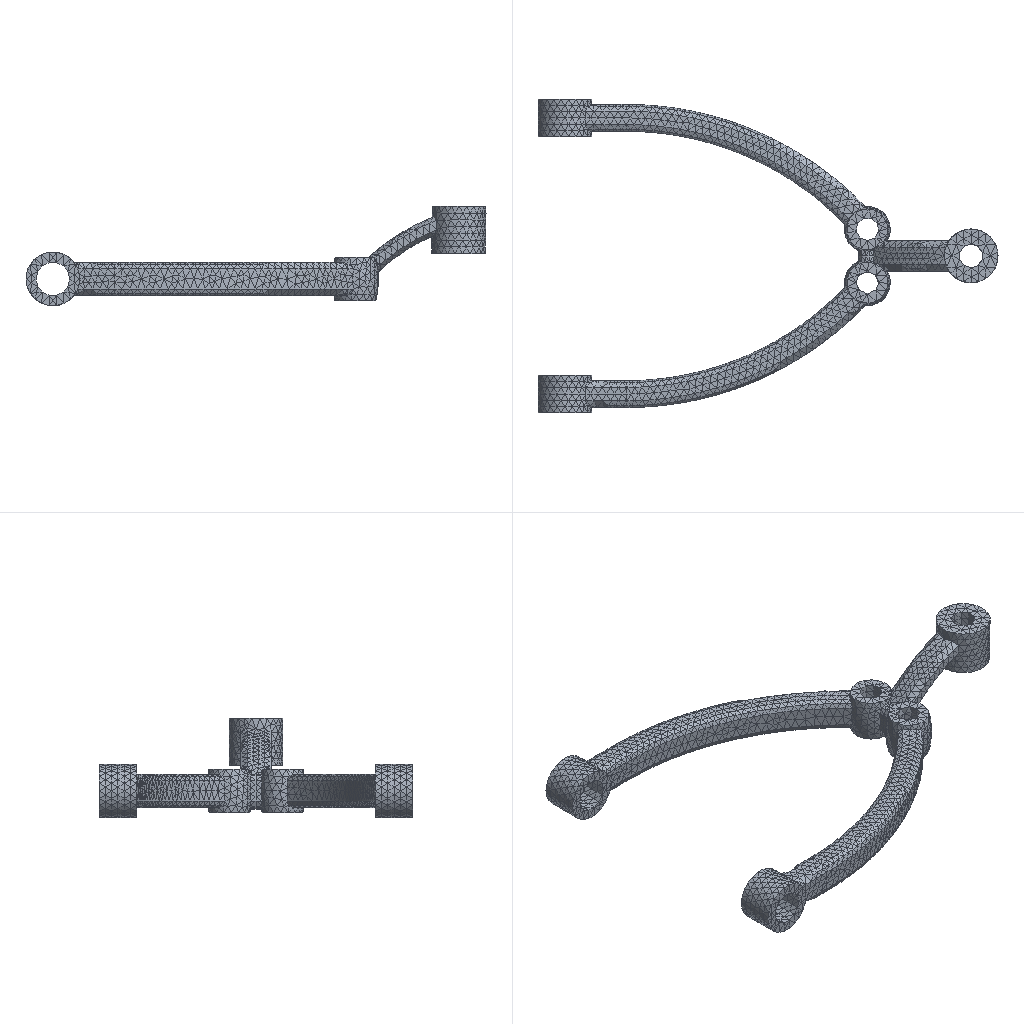Simulation study | nx simcenter
Set-up summary:
category,name,step,type,value,unit,region
solver,nx_nastran (Simcenter)
units,not stated in the deck,,not stated
analysis,deck,,static,static
analysis,solution,,SOL,101
load_step,SUBCASE 1,1,SUBCASE,SPC=5 LOAD=101
load_step,requested,,,1
mesh,nodes,,,18622
mesh,elements,,,9899
element_type,CTETRA,,solid,9899
load,nodal force total,,FX,0.0,model units
load,nodal force total,,FY,-2000,model units
load,nodal force total,,FZ,0.0,model units
load,load commands in deck,,count,261
bc,support commands in deck,,count,597
analysis,NX solution 0,,Structural,SESTATIC 101 - Single Constraint
analysis,NX solution 0,,Structural,SESTATIC 101 - Single Constraint
check,setup vs results,,match,every grid point's frame and coordinates and every element id; grid points of CTETRA elements
Nastran input file, long lists of numbers shortened:
$*$$$$$$$$$$$$$$$$$$$$$$$$$$$$$$$$$$$$$$$$$$$$$$$$$$$$$$$$$$$$$$$$$
$*
$*                    Simcenter v2412.0.0.1700 Translator
$*                    for Simcenter Nastran version 2412.0
$ (40 more lines like these left out)
ID,NASTRAN,8_fem1_sim1-solution_1
SOL 101
CEND
$*
$*$$$$$$$$$$$$$$$$$$$$$$$$$$$$$$$$$$$
$*
$* CASE CONTROL
$*
$*$$$$$$$$$$$$$$$$$$$$$$$$$$$$$$$$$$$
$*
ECHO = NONE
TEMP(INIT) = 1
OUTPUT
DISPLACEMENT(PLOT,REAL) = ALL
SPCFORCES(PLOT,REAL) = ALL
STRESS(PLOT,REAL,VONMISES,CENTER) = ALL
$*  Step: Subcase - Statics 1
SUBCASE 1
  LABEL = Subcase - Statics 1
  LOAD = 101
  SPC = 5
$*
$*$$$$$$$$$$$$$$$$$$$$$$$$$$$$$$$$$$$
$*
$* BULK DATA
$*
$*$$$$$$$$$$$$$$$$$$$$$$$$$$$$$$$$$$$
$*
BEGIN BULK
$*
$* PARAM CARDS
$*
PARAM      K6ROT100.0000
PARAM     OIBULK     YES
PARAM    OMACHPR     YES
PARAM       POST      -2
PARAM    POSTEXT     YES
PARAM    UNITSYS  LBF-IN
$*
$* GRID CARDS
$*
GRID*                  1               09.9999916553E-015.8399996758E+00+
*       -1.000000012E-07               0
GRID*                  2               09.9999439716E-01-5.839999676E+00+
*       -2.500006246E-07               0
$ (37240 more lines like these left out)
$*
$* ELEMENT CARDS
$*
$*  Mesh Collector: Solid(1)
$*  Mesh: 3d_mesh(1)
CTETRA         1       1    3591   10277    3604   10278   10788   10789+
+           3703   10790   10791   10792
CTETRA         2       1      20    3604   10277   10278   10793   10789+
+          10794   10795   10792   10791
$ (19794 more lines like these left out)
$*
$* PROPERTY CARDS
$*
$*  Property: PSOLID1::8_fem1::[2]
PSOLID         1       1       0                           SMECH
$*
$* MATERIAL CARDS
$*
$*  Material: Iron_Cast_G60::8_fem1::[1]
MAT1           12.2916+7        0.2500006.6904-46.0000-6
$*
$* LOAD AND CONSTRAINT CARDS
$*
$*  Solver Set: Temperature Set - Initial/Stress Free Temperature
TEMPD          1 37.0000
$*  Load: Force(1)
FORCE          2     184       0 18.9512  0.00001.000000  0.0000
FORCE          2     185       0 21.2272  0.00001.000000  0.0000
FORCE          2     186       0 19.9404  0.00001.000000  0.0000
FORCE          2     187       0 37.2688  0.00001.000000  0.0000
$ (98 more lines like these left out)
$*  Load: Force(2)
FORCE          3     141       0 28.4268  0.0000-1.00000  0.0000
FORCE          3     142       0 31.8408  0.0000-1.00000  0.0000
FORCE          3     143       0 56.2283  0.0000-1.00000  0.0000
FORCE          3     144       0 55.9033  0.0000-1.00000  0.0000
$ (98 more lines like these left out)
$*  Load: Pressure(1)
PLOAD4         4     149 20.0000                            1945    9158
PLOAD4         4     151 20.0000                            9328    9159
PLOAD4         4     304 20.0000                            2375    9497
PLOAD4         4     742 20.0000                            2368    9430
$ (52 more lines like these left out)
$*  Constraint: Fixed(1)
SPC            5      60  123456  0.0000
SPC            5      61  123456  0.0000
SPC            5      68  123456  0.0000
SPC            5      73  123456  0.0000
$ (593 more lines like these left out)
LOAD         1011.0000001.000000       21.000000       31.000000       4
ENDDATA 40df862b
Results summary:
result,analysis,,,static
result,last_loadstep,,,1
result,primary field,,,displacements
result,max displacement,,,1.742,model units
result,reaction total,,FX,0.5013,model units
result,reaction total,,FY,2000.085,model units
result,reaction total,,FZ,50.295,model units
result,NX solution 0,,loadcases,1,in
result,NX solution 0,,loadcases